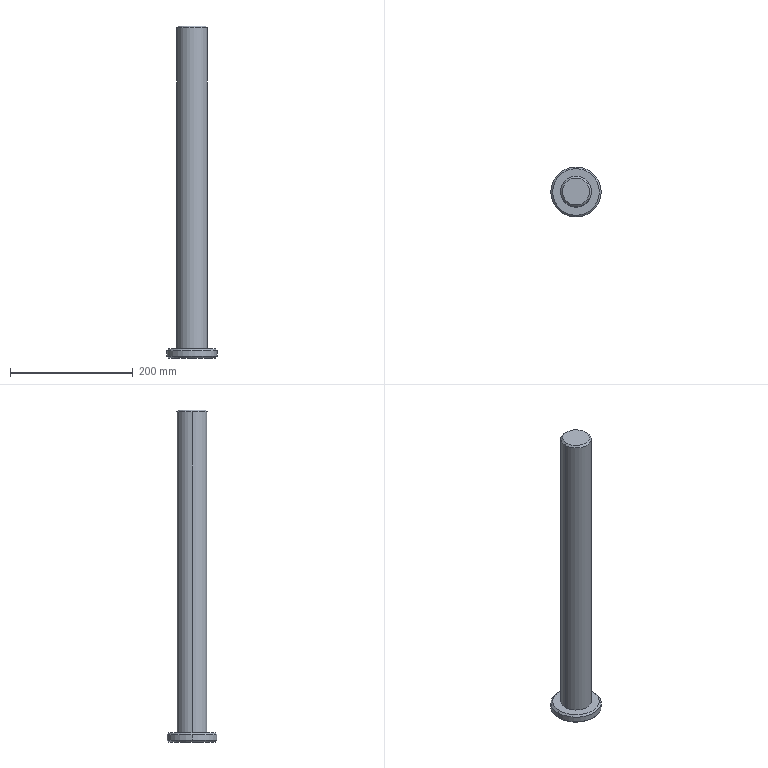Part | SolidWorks | features Chamfer 1, Extrusion 1, ICE 1 | 1 solid | 13 faces | box 82 x 82 x 541 mm | volume 1109073 mm3 | cone 6 | cylinder 4 | plane 3 | commonest cylinder face diameters 50 x2 82 x2
STEP:
#1=CARTESIAN_POINT('',(22.,0.,526.));
#2=VERTEX_POINT('',#1);
#3=CARTESIAN_POINT('',(-22.,0.,526.));
#4=VERTEX_POINT('',#3);
#5=CARTESIAN_POINT('',(0.,0.,526.));
#6=DIRECTION('',(0.,0.,1.));
#7=DIRECTION('',(1.,0.,0.));
#8=AXIS2_PLACEMENT_3D('',#5,#6,#7);
#9=CIRCLE('',#8,22.);
#10=EDGE_CURVE('',#2,#4,#9,.T.);
#11=ORIENTED_EDGE('',*,*,#10,.F.);
#12=CARTESIAN_POINT('',(25.,0.,523.));
#13=VERTEX_POINT('',#12);
#14=CARTESIAN_POINT('',(22.,0.,526.));
#15=DIRECTION('',(0.7071,0.,-0.7071));
#16=VECTOR('',#15,1000.);
#17=LINE('',#14,#16);
#18=EDGE_CURVE('',#2,#13,#17,.T.);
#19=ORIENTED_EDGE('',*,*,#18,.T.);
#20=CARTESIAN_POINT('',(-25.,0.,523.));
#21=VERTEX_POINT('',#20);
#22=CARTESIAN_POINT('',(0.,0.,523.));
#23=DIRECTION('',(0.,0.,-1.));
#24=DIRECTION('',(1.,0.,0.));
#25=AXIS2_PLACEMENT_3D('',#22,#23,#24);
#26=CIRCLE('',#25,25.);
#27=EDGE_CURVE('',#21,#13,#26,.T.);
#28=ORIENTED_EDGE('',*,*,#27,.F.);
#29=CARTESIAN_POINT('',(-22.,0.,526.));
#30=DIRECTION('',(-0.7071,0.,-0.7071));
#31=VECTOR('',#30,1000.);
#32=LINE('',#29,#31);
#33=EDGE_CURVE('',#4,#21,#32,.T.);
#34=ORIENTED_EDGE('',*,*,#33,.F.);
#35=EDGE_LOOP('',(#11,#19,#28,#34));
#36=FACE_OUTER_BOUND('',#35,.T.);
#37=CARTESIAN_POINT('',(0.,0.,526.));
#38=DIRECTION('',(0.,0.,-1.));
#39=DIRECTION('',(-1.,0.,0.));
#40=AXIS2_PLACEMENT_3D('',#37,#38,#39);
#41=CONICAL_SURFACE('',#40,22.,0.7854);
#42=ADVANCED_FACE('',(#36),#41,.T.);
#43=CARTESIAN_POINT('',(-38.,0.,-15.));
#44=VERTEX_POINT('',#43);
#45=CARTESIAN_POINT('',(38.,0.,-15.));
#46=VERTEX_POINT('',#45);
#47=CARTESIAN_POINT('',(0.,0.,-15.));
#48=DIRECTION('',(0.,0.,-1.));
#49=DIRECTION('',(-1.,0.,0.));
#50=AXIS2_PLACEMENT_3D('',#47,#48,#49);
#51=CIRCLE('',#50,38.);
#52=EDGE_CURVE('',#44,#46,#51,.T.);
#53=ORIENTED_EDGE('',*,*,#52,.F.);
#54=CARTESIAN_POINT('',(-41.,0.,-12.));
#55=VERTEX_POINT('',#54);
#56=CARTESIAN_POINT('',(-38.,0.,-15.));
#57=DIRECTION('',(-0.7071,0.,0.7071));
#58=VECTOR('',#57,1000.);
#59=LINE('',#56,#58);
#60=EDGE_CURVE('',#44,#55,#59,.T.);
#61=ORIENTED_EDGE('',*,*,#60,.T.);
#62=CARTESIAN_POINT('',(41.,0.,-12.));
#63=VERTEX_POINT('',#62);
#64=CARTESIAN_POINT('',(0.,0.,-12.));
#65=DIRECTION('',(0.,0.,1.));
#66=DIRECTION('',(-1.,0.,0.));
#67=AXIS2_PLACEMENT_3D('',#64,#65,#66);
#68=CIRCLE('',#67,41.);
#69=EDGE_CURVE('',#63,#55,#68,.T.);
#70=ORIENTED_EDGE('',*,*,#69,.F.);
#71=CARTESIAN_POINT('',(38.,0.,-15.));
#72=DIRECTION('',(0.7071,0.,0.7071));
#73=VECTOR('',#72,1000.);
#74=LINE('',#71,#73);
#75=EDGE_CURVE('',#46,#63,#74,.T.);
#76=ORIENTED_EDGE('',*,*,#75,.F.);
#77=EDGE_LOOP('',(#53,#61,#70,#76));
#78=FACE_OUTER_BOUND('',#77,.T.);
#79=CARTESIAN_POINT('',(0.,0.,-15.));
#80=DIRECTION('',(0.,0.,1.));
#81=DIRECTION('',(1.,0.,0.));
#82=AXIS2_PLACEMENT_3D('',#79,#80,#81);
#83=CONICAL_SURFACE('',#82,38.,0.7854);
#84=ADVANCED_FACE('',(#78),#83,.T.);
#85=CARTESIAN_POINT('',(38.,0.,0.));
#86=VERTEX_POINT('',#85);
#87=CARTESIAN_POINT('',(-38.,0.,0.));
#88=VERTEX_POINT('',#87);
#89=CARTESIAN_POINT('',(0.,0.,0.));
#90=DIRECTION('',(0.,0.,1.));
#91=DIRECTION('',(-1.,0.,0.));
#92=AXIS2_PLACEMENT_3D('',#89,#90,#91);
#93=CIRCLE('',#92,38.);
#94=EDGE_CURVE('',#86,#88,#93,.T.);
#95=ORIENTED_EDGE('',*,*,#94,.F.);
#96=CARTESIAN_POINT('',(41.,0.,-3.));
#97=VERTEX_POINT('',#96);
#98=CARTESIAN_POINT('',(41.,0.,-3.));
#99=DIRECTION('',(0.7071,0.,-0.7071));
#100=VECTOR('',#99,1000.);
#101=LINE('',#98,#100);
#102=EDGE_CURVE('',#86,#97,#101,.T.);
#103=ORIENTED_EDGE('',*,*,#102,.T.);
#104=CARTESIAN_POINT('',(-41.,0.,-3.));
#105=VERTEX_POINT('',#104);
#106=CARTESIAN_POINT('',(0.,0.,-3.));
#107=DIRECTION('',(0.,0.,-1.));
#108=DIRECTION('',(-1.,0.,0.));
#109=AXIS2_PLACEMENT_3D('',#106,#107,#108);
#110=CIRCLE('',#109,41.);
#111=EDGE_CURVE('',#105,#97,#110,.T.);
#112=ORIENTED_EDGE('',*,*,#111,.F.);
#113=CARTESIAN_POINT('',(-41.,0.,-3.));
#114=DIRECTION('',(-0.7071,0.,-0.7071));
#115=VECTOR('',#114,1000.);
#116=LINE('',#113,#115);
#117=EDGE_CURVE('',#88,#105,#116,.T.);
#118=ORIENTED_EDGE('',*,*,#117,.F.);
#119=EDGE_LOOP('',(#95,#103,#112,#118));
#120=FACE_OUTER_BOUND('',#119,.T.);
#121=CARTESIAN_POINT('',(0.,0.,-3.));
#122=DIRECTION('',(0.,0.,-1.));
#123=DIRECTION('',(-1.,0.,0.));
#124=AXIS2_PLACEMENT_3D('',#121,#122,#123);
#125=CONICAL_SURFACE('',#124,41.,0.7854);
#126=ADVANCED_FACE('',(#120),#125,.T.);
#127=ORIENTED_EDGE('',*,*,#69,.T.);
#128=CARTESIAN_POINT('',(-41.,0.,-15.));
#129=DIRECTION('',(0.,0.,1.));
#130=VECTOR('',#129,1000.);
#131=LINE('',#128,#130);
#132=EDGE_CURVE('',#55,#105,#131,.T.);
#133=ORIENTED_EDGE('',*,*,#132,.T.);
#134=ORIENTED_EDGE('',*,*,#111,.T.);
#135=CARTESIAN_POINT('',(41.,0.,-15.));
#136=DIRECTION('',(0.,0.,1.));
#137=VECTOR('',#136,1000.);
#138=LINE('',#135,#137);
#139=EDGE_CURVE('',#63,#97,#138,.T.);
#140=ORIENTED_EDGE('',*,*,#139,.F.);
#141=EDGE_LOOP('',(#127,#133,#134,#140));
#142=FACE_OUTER_BOUND('',#141,.T.);
#143=CARTESIAN_POINT('',(0.,0.,-15.));
#144=DIRECTION('',(0.,0.,1.));
#145=DIRECTION('',(1.,0.,0.));
#146=AXIS2_PLACEMENT_3D('',#143,#144,#145);
#147=CYLINDRICAL_SURFACE('',#146,41.);
#148=ADVANCED_FACE('',(#142),#147,.T.);
#149=ORIENTED_EDGE('',*,*,#27,.T.);
#150=CARTESIAN_POINT('',(25.,0.,0.));
#151=VERTEX_POINT('',#150);
#152=CARTESIAN_POINT('',(25.,0.,526.));
#153=DIRECTION('',(0.,0.,-1.));
#154=VECTOR('',#153,1000.);
#155=LINE('',#152,#154);
#156=EDGE_CURVE('',#13,#151,#155,.T.);
#157=ORIENTED_EDGE('',*,*,#156,.T.);
#158=CARTESIAN_POINT('',(-25.,0.,0.));
#159=VERTEX_POINT('',#158);
#160=CARTESIAN_POINT('',(0.,0.,0.));
#161=DIRECTION('',(0.,0.,1.));
#162=DIRECTION('',(1.,0.,0.));
#163=AXIS2_PLACEMENT_3D('',#160,#161,#162);
#164=CIRCLE('',#163,25.);
#165=EDGE_CURVE('',#151,#159,#164,.T.);
#166=ORIENTED_EDGE('',*,*,#165,.T.);
#167=CARTESIAN_POINT('',(-25.,0.,526.));
#168=DIRECTION('',(0.,0.,-1.));
#169=VECTOR('',#168,1000.);
#170=LINE('',#167,#169);
#171=EDGE_CURVE('',#21,#159,#170,.T.);
#172=ORIENTED_EDGE('',*,*,#171,.F.);
#173=EDGE_LOOP('',(#149,#157,#166,#172));
#174=FACE_OUTER_BOUND('',#173,.T.);
#175=CARTESIAN_POINT('',(0.,0.,526.));
#176=DIRECTION('',(0.,0.,-1.));
#177=DIRECTION('',(-1.,0.,0.));
#178=AXIS2_PLACEMENT_3D('',#175,#176,#177);
#179=CYLINDRICAL_SURFACE('',#178,25.);
#180=ADVANCED_FACE('',(#174),#179,.T.);
#181=ORIENTED_EDGE('',*,*,#156,.F.);
#182=CARTESIAN_POINT('',(0.,0.,523.));
#183=DIRECTION('',(0.,0.,-1.));
#184=DIRECTION('',(1.,0.,0.));
#185=AXIS2_PLACEMENT_3D('',#182,#183,#184);
#186=CIRCLE('',#185,25.);
#187=EDGE_CURVE('',#13,#21,#186,.T.);
#188=ORIENTED_EDGE('',*,*,#187,.T.);
#189=ORIENTED_EDGE('',*,*,#171,.T.);
#190=CARTESIAN_POINT('',(0.,0.,0.));
#191=DIRECTION('',(0.,0.,1.));
#192=DIRECTION('',(1.,0.,0.));
#193=AXIS2_PLACEMENT_3D('',#190,#191,#192);
#194=CIRCLE('',#193,25.);
#195=EDGE_CURVE('',#159,#151,#194,.T.);
#196=ORIENTED_EDGE('',*,*,#195,.T.);
#197=EDGE_LOOP('',(#181,#188,#189,#196));
#198=FACE_OUTER_BOUND('',#197,.T.);
#199=CARTESIAN_POINT('',(0.,0.,526.));
#200=DIRECTION('',(0.,0.,-1.));
#201=DIRECTION('',(-1.,0.,0.));
#202=AXIS2_PLACEMENT_3D('',#199,#200,#201);
#203=CYLINDRICAL_SURFACE('',#202,25.);
#204=ADVANCED_FACE('',(#198),#203,.T.);
#205=CARTESIAN_POINT('',(0.,0.,526.));
#206=DIRECTION('',(0.,0.,1.));
#207=DIRECTION('',(1.,0.,0.));
#208=AXIS2_PLACEMENT_3D('',#205,#206,#207);
#209=CIRCLE('',#208,22.);
#210=EDGE_CURVE('',#4,#2,#209,.T.);
#211=ORIENTED_EDGE('',*,*,#210,.T.);
#212=ORIENTED_EDGE('',*,*,#10,.T.);
#213=EDGE_LOOP('',(#211,#212));
#214=FACE_OUTER_BOUND('',#213,.T.);
#215=CARTESIAN_POINT('',(0.,0.,526.));
#216=DIRECTION('',(0.,0.,1.));
#217=DIRECTION('',(1.,0.,0.));
#218=AXIS2_PLACEMENT_3D('',#215,#216,#217);
#219=PLANE('',#218);
#220=ADVANCED_FACE('',(#214),#219,.T.);
#221=ORIENTED_EDGE('',*,*,#132,.F.);
#222=CARTESIAN_POINT('',(0.,0.,-12.));
#223=DIRECTION('',(0.,0.,1.));
#224=DIRECTION('',(-1.,0.,0.));
#225=AXIS2_PLACEMENT_3D('',#222,#223,#224);
#226=CIRCLE('',#225,41.);
#227=EDGE_CURVE('',#55,#63,#226,.T.);
#228=ORIENTED_EDGE('',*,*,#227,.T.);
#229=ORIENTED_EDGE('',*,*,#139,.T.);
#230=CARTESIAN_POINT('',(0.,0.,-3.));
#231=DIRECTION('',(0.,0.,-1.));
#232=DIRECTION('',(-1.,0.,0.));
#233=AXIS2_PLACEMENT_3D('',#230,#231,#232);
#234=CIRCLE('',#233,41.);
#235=EDGE_CURVE('',#97,#105,#234,.T.);
#236=ORIENTED_EDGE('',*,*,#235,.T.);
#237=EDGE_LOOP('',(#221,#228,#229,#236));
#238=FACE_OUTER_BOUND('',#237,.T.);
#239=CARTESIAN_POINT('',(0.,0.,-15.));
#240=DIRECTION('',(0.,0.,1.));
#241=DIRECTION('',(1.,0.,0.));
#242=AXIS2_PLACEMENT_3D('',#239,#240,#241);
#243=CYLINDRICAL_SURFACE('',#242,41.);
#244=ADVANCED_FACE('',(#238),#243,.T.);
#245=CARTESIAN_POINT('',(0.,0.,-15.));
#246=DIRECTION('',(0.,0.,-1.));
#247=DIRECTION('',(-1.,0.,0.));
#248=AXIS2_PLACEMENT_3D('',#245,#246,#247);
#249=CIRCLE('',#248,38.);
#250=EDGE_CURVE('',#46,#44,#249,.T.);
#251=ORIENTED_EDGE('',*,*,#250,.T.);
#252=ORIENTED_EDGE('',*,*,#52,.T.);
#253=EDGE_LOOP('',(#251,#252));
#254=FACE_OUTER_BOUND('',#253,.T.);
#255=CARTESIAN_POINT('',(0.,0.,-15.));
#256=DIRECTION('',(0.,0.,-1.));
#257=DIRECTION('',(-1.,0.,0.));
#258=AXIS2_PLACEMENT_3D('',#255,#256,#257);
#259=PLANE('',#258);
#260=ADVANCED_FACE('',(#254),#259,.T.);
#261=CARTESIAN_POINT('',(0.,0.,0.));
#262=DIRECTION('',(0.,0.,1.));
#263=DIRECTION('',(-1.,0.,0.));
#264=AXIS2_PLACEMENT_3D('',#261,#262,#263);
#265=CIRCLE('',#264,38.);
#266=EDGE_CURVE('',#88,#86,#265,.T.);
#267=ORIENTED_EDGE('',*,*,#266,.T.);
#268=ORIENTED_EDGE('',*,*,#94,.T.);
#269=EDGE_LOOP('',(#267,#268));
#270=FACE_OUTER_BOUND('',#269,.T.);
#271=ORIENTED_EDGE('',*,*,#195,.F.);
#272=ORIENTED_EDGE('',*,*,#165,.F.);
#273=EDGE_LOOP('',(#271,#272));
#274=FACE_BOUND('',#273,.T.);
#275=CARTESIAN_POINT('',(0.,0.,0.));
#276=DIRECTION('',(0.,0.,-1.));
#277=DIRECTION('',(-1.,0.,0.));
#278=AXIS2_PLACEMENT_3D('',#275,#276,#277);
#279=PLANE('',#278);
#280=ADVANCED_FACE('',(#270,#274),#279,.F.);
#281=ORIENTED_EDGE('',*,*,#102,.F.);
#282=ORIENTED_EDGE('',*,*,#266,.F.);
#283=ORIENTED_EDGE('',*,*,#117,.T.);
#284=ORIENTED_EDGE('',*,*,#235,.F.);
#285=EDGE_LOOP('',(#281,#282,#283,#284));
#286=FACE_OUTER_BOUND('',#285,.T.);
#287=CARTESIAN_POINT('',(0.,0.,-3.));
#288=DIRECTION('',(0.,0.,-1.));
#289=DIRECTION('',(-1.,0.,0.));
#290=AXIS2_PLACEMENT_3D('',#287,#288,#289);
#291=CONICAL_SURFACE('',#290,41.,0.7854);
#292=ADVANCED_FACE('',(#286),#291,.T.);
#293=ORIENTED_EDGE('',*,*,#60,.F.);
#294=ORIENTED_EDGE('',*,*,#250,.F.);
#295=ORIENTED_EDGE('',*,*,#75,.T.);
#296=ORIENTED_EDGE('',*,*,#227,.F.);
#297=EDGE_LOOP('',(#293,#294,#295,#296));
#298=FACE_OUTER_BOUND('',#297,.T.);
#299=CARTESIAN_POINT('',(0.,0.,-15.));
#300=DIRECTION('',(0.,0.,1.));
#301=DIRECTION('',(1.,0.,0.));
#302=AXIS2_PLACEMENT_3D('',#299,#300,#301);
#303=CONICAL_SURFACE('',#302,38.,0.7854);
#304=ADVANCED_FACE('',(#298),#303,.T.);
#305=ORIENTED_EDGE('',*,*,#18,.F.);
#306=ORIENTED_EDGE('',*,*,#210,.F.);
#307=ORIENTED_EDGE('',*,*,#33,.T.);
#308=ORIENTED_EDGE('',*,*,#187,.F.);
#309=EDGE_LOOP('',(#305,#306,#307,#308));
#310=FACE_OUTER_BOUND('',#309,.T.);
#311=CARTESIAN_POINT('',(0.,0.,526.));
#312=DIRECTION('',(0.,0.,-1.));
#313=DIRECTION('',(-1.,0.,0.));
#314=AXIS2_PLACEMENT_3D('',#311,#312,#313);
#315=CONICAL_SURFACE('',#314,22.,0.7854);
#316=ADVANCED_FACE('',(#310),#315,.T.);
#317=CLOSED_SHELL('',(#42,#84,#126,#148,#180,#204,#220,#244,#260,#280,#292,#304,#316));
#318=MANIFOLD_SOLID_BREP('',#317);
#319=CARTESIAN_POINT('',(0.,0.,0.));
#320=DIRECTION('',(0.,0.,1.));
#321=DIRECTION('',(1.,0.,0.));
#322=AXIS2_PLACEMENT_3D('',#319,#320,#321);
#323=(LENGTH_UNIT()NAMED_UNIT(*)SI_UNIT(.MILLI.,.METRE.));
#324=UNCERTAINTY_MEASURE_WITH_UNIT(LENGTH_MEASURE(0.00001),#323,'','');
#325=(NAMED_UNIT(*)PLANE_ANGLE_UNIT()SI_UNIT($,.RADIAN.));
#326=(NAMED_UNIT(*)SI_UNIT($,.STERADIAN.)SOLID_ANGLE_UNIT());
#327=(GEOMETRIC_REPRESENTATION_CONTEXT(3)GLOBAL_UNCERTAINTY_ASSIGNED_CONTEXT((#324))GLOBAL_UNIT_ASSIGNED_CONTEXT((#323,#325,#326))REPRESENTATION_CONTEXT('',''));
#328=ADVANCED_BREP_SHAPE_REPRESENTATION('',(#318,#322),#327);